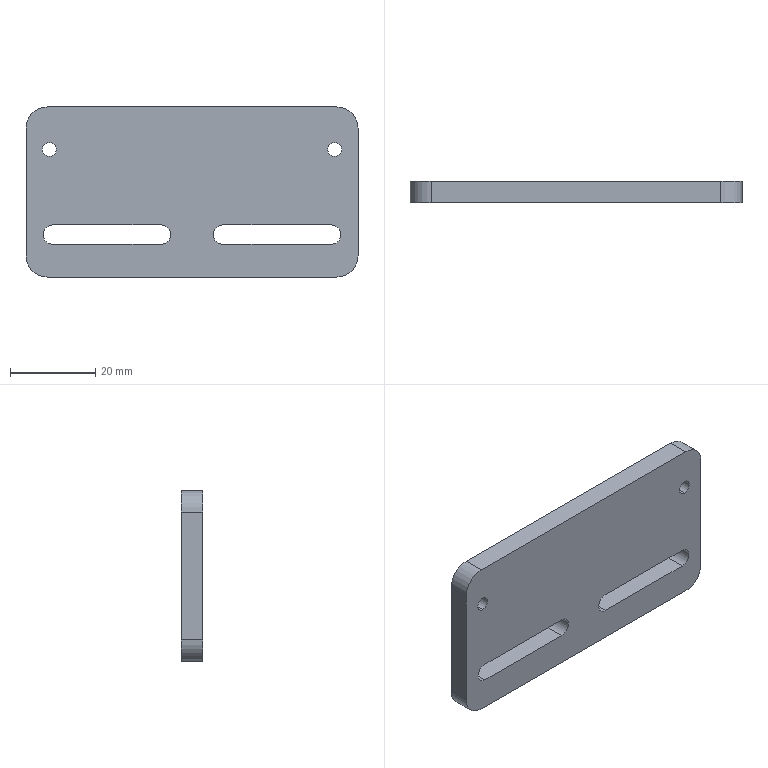Part | STEP file | energy chain mounting plate | 1 solid | 22 faces | box 78 x 5 x 40 mm | volume 14101 mm3 | cylinder 12 | plane 10 | commonest cylinder face diameters 3.3 x4 4.5 x4 10 x4